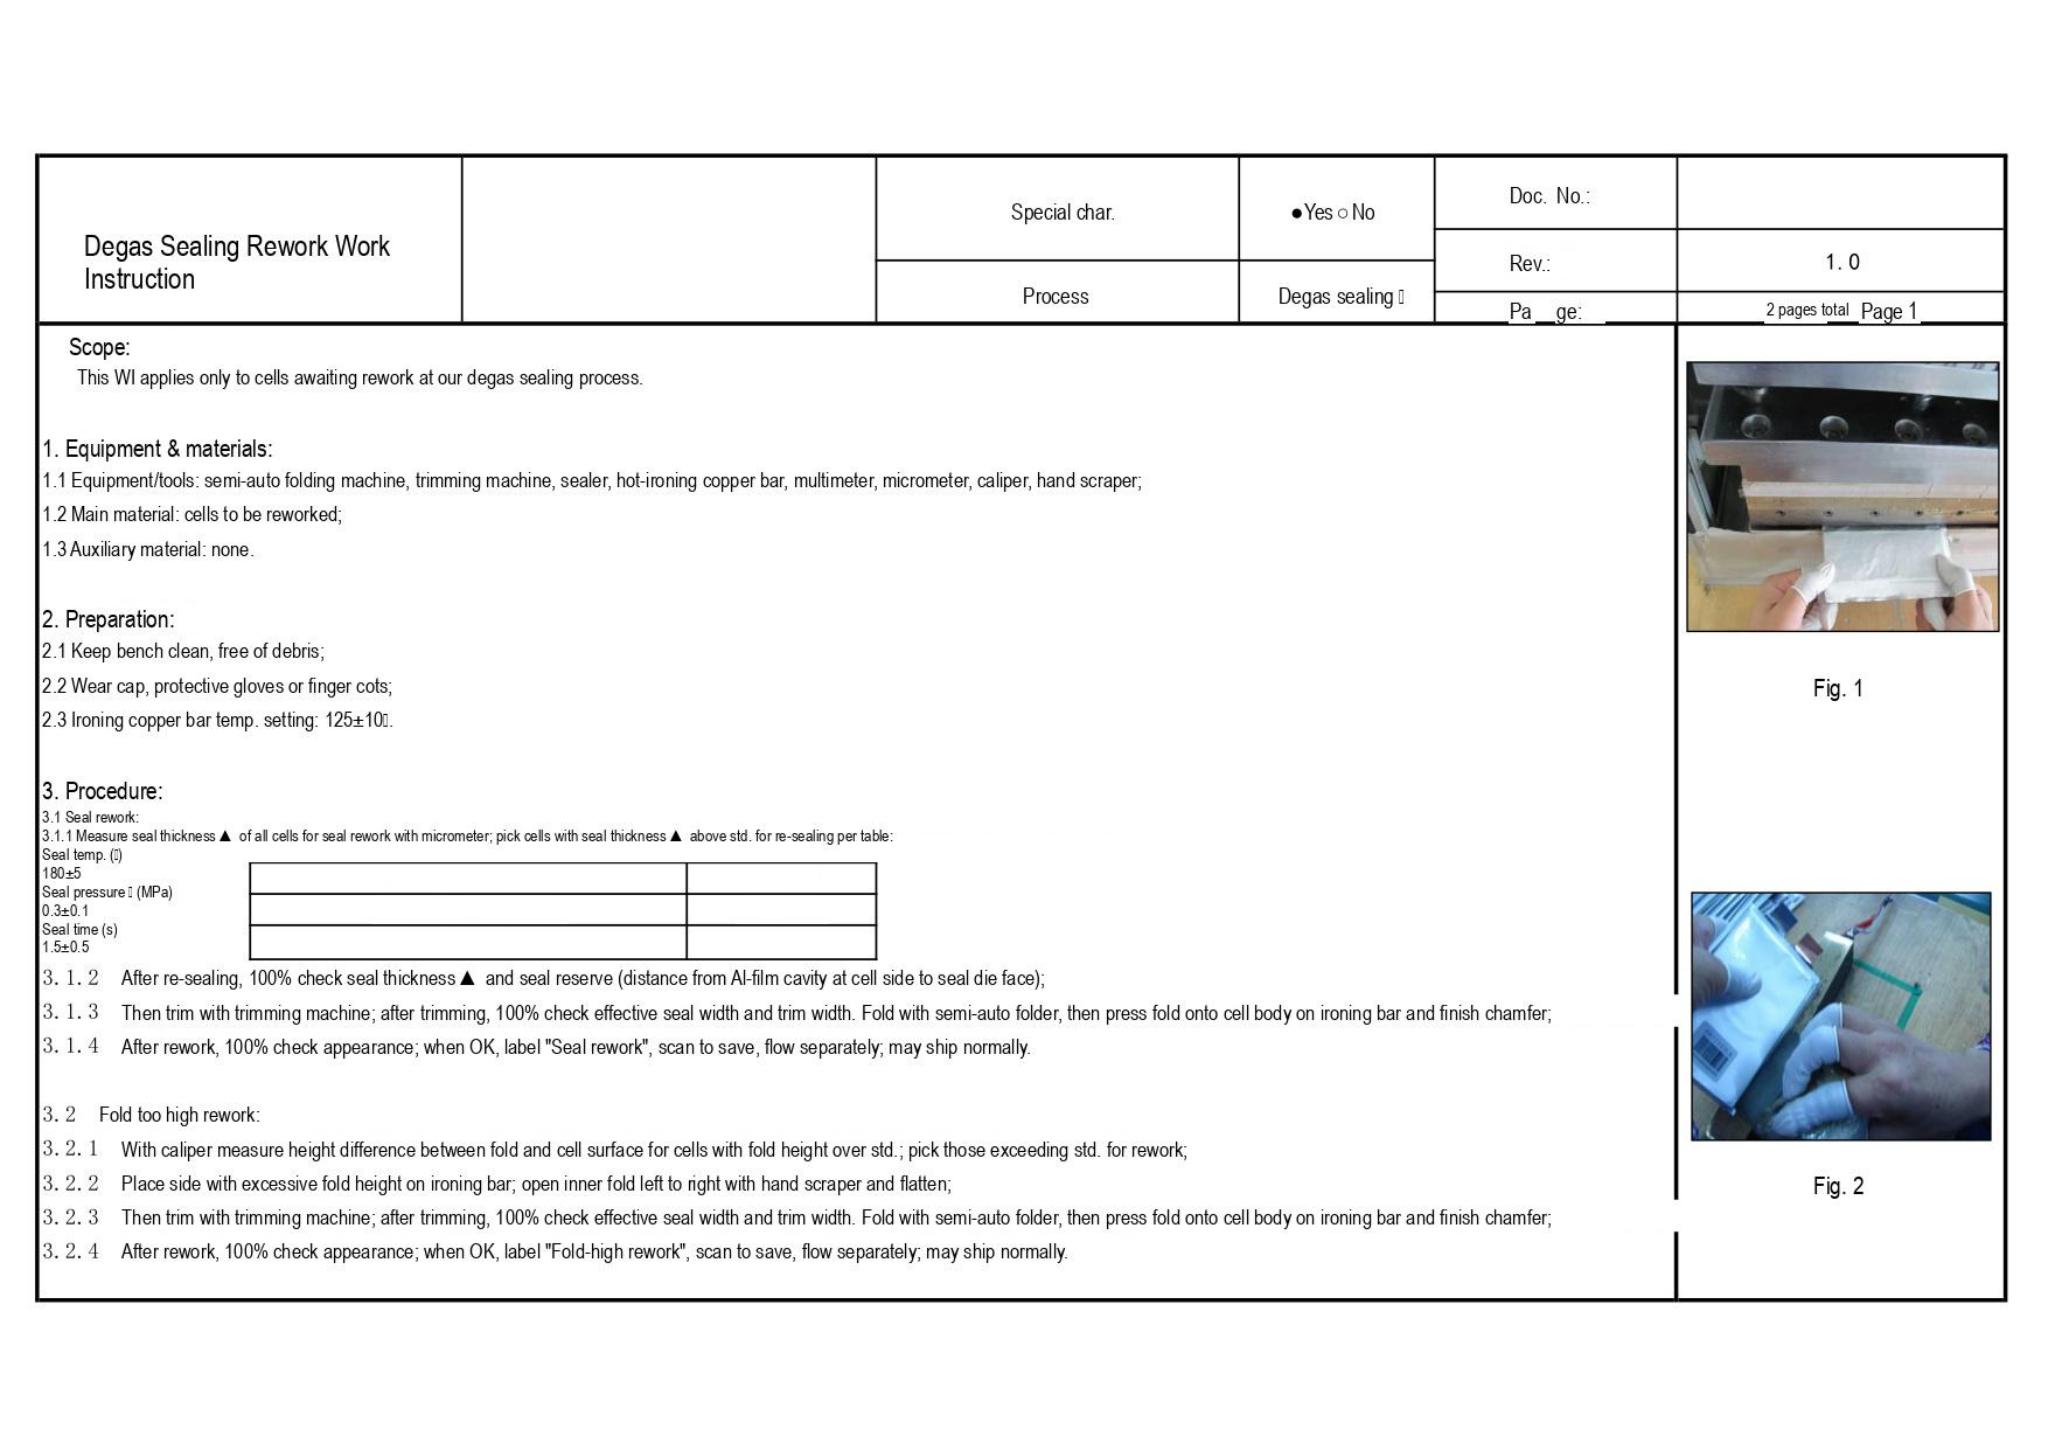| Degas Sealing Rework Work Instruction | | Special char. | ●Yes ○No | Doc. No.: | |
|---|---|---|---|---|---|
| | | | | Rev.: | 1. 0 |
| | | Process | Degas sealing | Pa ge: | 2 pages total Page 1 |

Scope:
This WI applies only to cells awaiting rework at our degas sealing process.

1. Equipment & materials:
1.1 Equipment/tools: semi-auto folding machine, trimming machine, sealer, hot-ironing copper bar, multimeter, micrometer, caliper, hand scraper;
1.2 Main material: cells to be reworked;
1.3 Auxiliary material: none.

2. Preparation:
2.1 Keep bench clean, free of debris;
2.2 Wear cap, protective gloves or finger cots;
2.3 Ironing copper bar temp. setting: 125±10.

3. Procedure:
3.1 Seal rework:
3.1.1 Measure seal thickness ▲ of all cells for seal rework with micrometer; pick cells with seal thickness ▲ above std. for re-sealing per table:
Seal temp. ()
180±5
Seal pressure (MPa)
0.3±0.1
Seal time (s)
1.5±0.5
3. 1. 2 After re-sealing, 100% check seal thickness ▲ and seal reserve (distance from Al-film cavity at cell side to seal die face);
3. 1. 3 Then trim with trimming machine; after trimming, 100% check effective seal width and trim width. Fold with semi-auto folder, then press fold onto cell body on ironing bar and finish chamfer;
3. 1. 4 After rework, 100% check appearance; when OK, label "Seal rework", scan to save, flow separately; may ship normally.

3. 2 Fold too high rework:
3. 2. 1 With caliper measure height difference between fold and cell surface for cells with fold height over std.; pick those exceeding std. for rework;
3. 2. 2 Place side with excessive fold height on ironing bar; open inner fold left to right with hand scraper and flatten;
3. 2. 3 Then trim with trimming machine; after trimming, 100% check effective seal width and trim width. Fold with semi-auto folder, then press fold onto cell body on ironing bar and finish chamfer;
3. 2. 4 After rework, 100% check appearance; when OK, label "Fold-high rework", scan to save, flow separately; may ship normally.

Fig. 1

Fig. 2
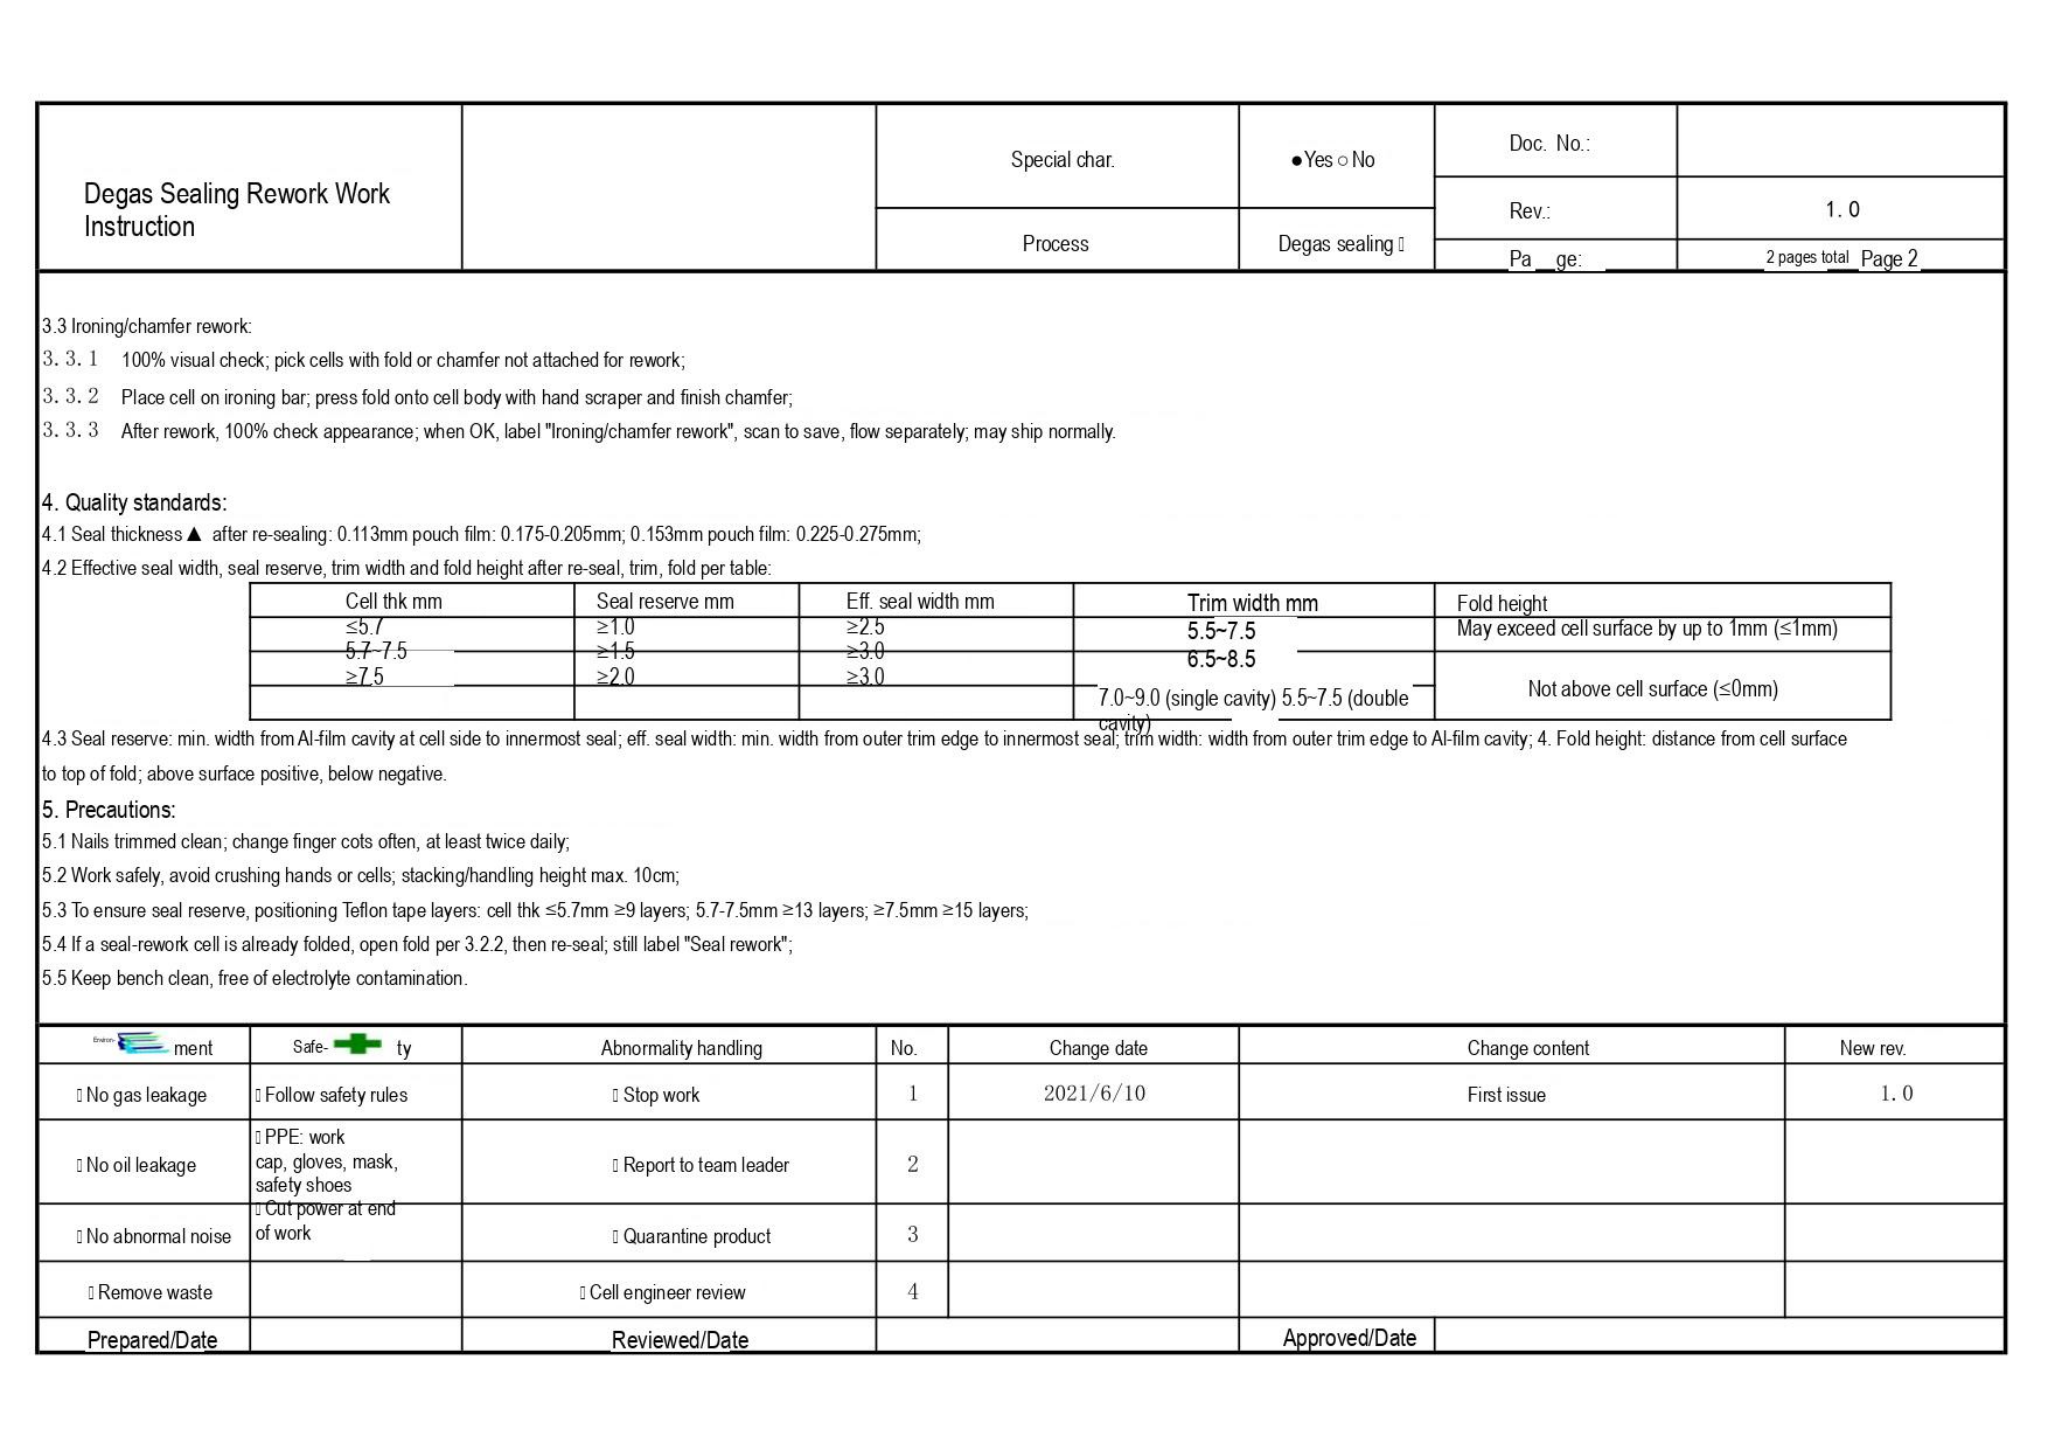| Degas Sealing Rework Work Instruction | | Special char. | ●Yes ○ No | Doc. No.: | |
|---|---|---|---|---|---|
| | | | | Rev.: | 1. 0 |
| | | Process | Degas sealing | Page: | 2 pages total Page 2 |

3.3 Ironing/chamfer rework:

3. 3. 1 100% visual check; pick cells with fold or chamfer not attached for rework;

3. 3. 2 Place cell on ironing bar; press fold onto cell body with hand scraper and finish chamfer;

3. 3. 3 After rework, 100% check appearance; when OK, label "Ironing/chamfer rework", scan to save, flow separately; may ship normally.

4. Quality standards:

4.1 Seal thickness ▲ after re-sealing: 0.113mm pouch film: 0.175-0.205mm; 0.153mm pouch film: 0.225-0.275mm;

4.2 Effective seal width, seal reserve, trim width and fold height after re-seal, trim, fold per table:

| Cell thk mm | Seal reserve mm | Eff. seal width mm | Trim width mm | Fold height |
|---|---|---|---|---|
| ≤5.7 | ≥1.0 | ≥2.5 | 5.5~7.5 | May exceed cell surface by up to 1mm (≤1mm) |
| 5.7-7.5 | ≥1.5 | ≥3.0 | 6.5~8.5 | Not above cell surface (≤0mm) |
| ≥7.5 | ≥2.0 | ≥3.0 | 7.0~9.0 (single cavity) 5.5~7.5 (double cavity) | |

4.3 Seal reserve: min. width from Al-film cavity at cell side to innermost seal; eff. seal width: min. width from outer trim edge to innermost seal; trim width: width from outer trim edge to Al-film cavity; 4. Fold height: distance from cell surface to top of fold; above surface positive, below negative.

5. Precautions:

5.1 Nails trimmed clean; change finger cots often, at least twice daily;

5.2 Work safely, avoid crushing hands or cells; stacking/handling height max. 10cm;

5.3 To ensure seal reserve, positioning Teflon tape layers: cell thk ≤5.7mm ≥9 layers; 5.7-7.5mm ≥13 layers; ≥7.5mm ≥15 layers;

5.4 If a seal-rework cell is already folded, open fold per 3.2.2, then re-seal; still label "Seal rework";

5.5 Keep bench clean, free of electrolyte contamination.

| Environment | Safety | Abnormality handling | No. | Change date | Change content | New rev. |
|---|---|---|---|---|---|---|
| No gas leakage | Follow safety rules | Stop work | 1 | 2021/6/10 | First issue | 1. 0 |
| No oil leakage | PPE: work cap, gloves, mask, safety shoes | Report to team leader | 2 | | | |
| No abnormal noise | Cut power at end of work | Quarantine product | 3 | | | |
| Remove waste | | Cell engineer review | 4 | | | |
| Prepared/Date | | Reviewed/Date | | | Approved/Date | |